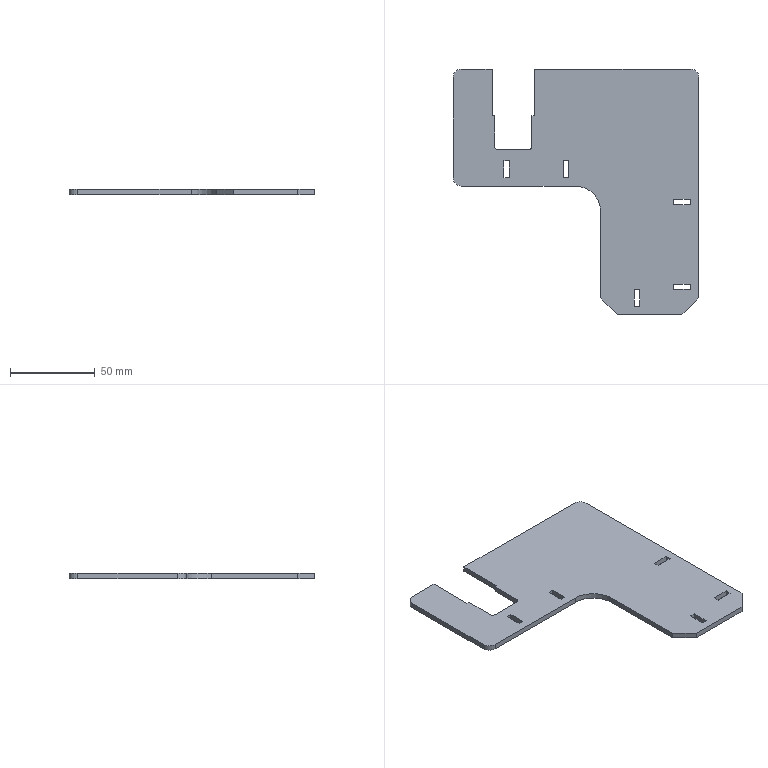Part | SolidWorks | features FlatPattern 1, SMBaseFlange 1, SheetMetal 1 | 1 solid | 44 faces | box 145 x 145 x 3.2 mm | volume 41790 mm3 | plane 38 | cylinder 6 | commonest cylinder face diameters 10 x3 4 x2 30 x1
STEP:
#1=CARTESIAN_POINT('',(-266.995,-106.198,3.2));
#2=VERTEX_POINT('',#1);
#3=CARTESIAN_POINT('',(-266.995,-133.698,3.2));
#4=VERTEX_POINT('',#3);
#5=CARTESIAN_POINT('',(-266.995,-133.698,3.2));
#6=DIRECTION('',(0.,-1.,0.));
#7=VECTOR('',#6,1000.);
#8=LINE('',#5,#7);
#9=EDGE_CURVE('',#2,#4,#8,.T.);
#10=ORIENTED_EDGE('',*,*,#9,.T.);
#11=CARTESIAN_POINT('',(-268.495,-133.698,3.2));
#12=VERTEX_POINT('',#11);
#13=CARTESIAN_POINT('',(-268.495,-133.698,3.2));
#14=DIRECTION('',(-1.,0.,0.));
#15=VECTOR('',#14,1000.);
#16=LINE('',#13,#15);
#17=EDGE_CURVE('',#4,#12,#16,.T.);
#18=ORIENTED_EDGE('',*,*,#17,.T.);
#19=CARTESIAN_POINT('',(-268.495,-151.698,3.2));
#20=VERTEX_POINT('',#19);
#21=CARTESIAN_POINT('',(-268.495,-151.698,3.2));
#22=DIRECTION('',(0.,-1.,0.));
#23=VECTOR('',#22,1000.);
#24=LINE('',#21,#23);
#25=EDGE_CURVE('',#12,#20,#24,.T.);
#26=ORIENTED_EDGE('',*,*,#25,.T.);
#27=CARTESIAN_POINT('',(-270.495,-153.698,3.2));
#28=VERTEX_POINT('',#27);
#29=CARTESIAN_POINT('',(-270.495,-151.698,3.2));
#30=DIRECTION('',(0.,0.,-1.));
#31=DIRECTION('',(1.,0.,0.));
#32=AXIS2_PLACEMENT_3D('',#29,#30,#31);
#33=CIRCLE('',#32,2.);
#34=EDGE_CURVE('',#20,#28,#33,.T.);
#35=ORIENTED_EDGE('',*,*,#34,.T.);
#36=CARTESIAN_POINT('',(-288.495,-153.698,3.2));
#37=VERTEX_POINT('',#36);
#38=CARTESIAN_POINT('',(-288.495,-153.698,3.2));
#39=DIRECTION('',(-1.,0.,0.));
#40=VECTOR('',#39,1000.);
#41=LINE('',#38,#40);
#42=EDGE_CURVE('',#28,#37,#41,.T.);
#43=ORIENTED_EDGE('',*,*,#42,.T.);
#44=CARTESIAN_POINT('',(-290.495,-151.698,3.2));
#45=VERTEX_POINT('',#44);
#46=CARTESIAN_POINT('',(-288.495,-151.698,3.2));
#47=DIRECTION('',(0.,0.,-1.));
#48=DIRECTION('',(1.,0.,0.));
#49=AXIS2_PLACEMENT_3D('',#46,#47,#48);
#50=CIRCLE('',#49,2.);
#51=EDGE_CURVE('',#37,#45,#50,.T.);
#52=ORIENTED_EDGE('',*,*,#51,.T.);
#53=CARTESIAN_POINT('',(-290.495,-133.698,3.2));
#54=VERTEX_POINT('',#53);
#55=CARTESIAN_POINT('',(-290.495,-133.698,3.2));
#56=DIRECTION('',(0.,1.,0.));
#57=VECTOR('',#56,1000.);
#58=LINE('',#55,#57);
#59=EDGE_CURVE('',#45,#54,#58,.T.);
#60=ORIENTED_EDGE('',*,*,#59,.T.);
#61=CARTESIAN_POINT('',(-291.995,-133.698,3.2));
#62=VERTEX_POINT('',#61);
#63=CARTESIAN_POINT('',(-291.995,-133.698,3.2));
#64=DIRECTION('',(-1.,0.,0.));
#65=VECTOR('',#64,1000.);
#66=LINE('',#63,#65);
#67=EDGE_CURVE('',#54,#62,#66,.T.);
#68=ORIENTED_EDGE('',*,*,#67,.T.);
#69=CARTESIAN_POINT('',(-291.995,-106.198,3.2));
#70=VERTEX_POINT('',#69);
#71=CARTESIAN_POINT('',(-291.995,-133.698,3.2));
#72=DIRECTION('',(0.,1.,0.));
#73=VECTOR('',#72,1000.);
#74=LINE('',#71,#73);
#75=EDGE_CURVE('',#62,#70,#74,.T.);
#76=ORIENTED_EDGE('',*,*,#75,.T.);
#77=CARTESIAN_POINT('',(-309.995,-106.198,3.2));
#78=VERTEX_POINT('',#77);
#79=CARTESIAN_POINT('',(-309.995,-106.198,3.2));
#80=DIRECTION('',(-1.,0.,0.));
#81=VECTOR('',#80,1000.);
#82=LINE('',#79,#81);
#83=EDGE_CURVE('',#70,#78,#82,.T.);
#84=ORIENTED_EDGE('',*,*,#83,.T.);
#85=CARTESIAN_POINT('',(-314.995,-111.198,3.2));
#86=VERTEX_POINT('',#85);
#87=CARTESIAN_POINT('',(-309.995,-111.198,3.2));
#88=DIRECTION('',(0.,0.,1.));
#89=DIRECTION('',(-1.,0.,0.));
#90=AXIS2_PLACEMENT_3D('',#87,#88,#89);
#91=CIRCLE('',#90,5.);
#92=EDGE_CURVE('',#78,#86,#91,.T.);
#93=ORIENTED_EDGE('',*,*,#92,.T.);
#94=CARTESIAN_POINT('',(-314.995,-170.198,3.2));
#95=VERTEX_POINT('',#94);
#96=CARTESIAN_POINT('',(-314.995,-170.198,3.2));
#97=DIRECTION('',(0.,-1.,0.));
#98=VECTOR('',#97,1000.);
#99=LINE('',#96,#98);
#100=EDGE_CURVE('',#86,#95,#99,.T.);
#101=ORIENTED_EDGE('',*,*,#100,.T.);
#102=CARTESIAN_POINT('',(-309.995,-175.198,3.2));
#103=VERTEX_POINT('',#102);
#104=CARTESIAN_POINT('',(-309.995,-170.198,3.2));
#105=DIRECTION('',(0.,0.,1.));
#106=DIRECTION('',(-1.,0.,0.));
#107=AXIS2_PLACEMENT_3D('',#104,#105,#106);
#108=CIRCLE('',#107,5.);
#109=EDGE_CURVE('',#95,#103,#108,.T.);
#110=ORIENTED_EDGE('',*,*,#109,.T.);
#111=CARTESIAN_POINT('',(-242.995,-175.198,3.2));
#112=VERTEX_POINT('',#111);
#113=CARTESIAN_POINT('',(-242.995,-175.198,3.2));
#114=DIRECTION('',(1.,0.,0.));
#115=VECTOR('',#114,1000.);
#116=LINE('',#113,#115);
#117=EDGE_CURVE('',#103,#112,#116,.T.);
#118=ORIENTED_EDGE('',*,*,#117,.T.);
#119=CARTESIAN_POINT('',(-227.995,-190.198,3.2));
#120=VERTEX_POINT('',#119);
#121=CARTESIAN_POINT('',(-242.995,-190.198,3.2));
#122=DIRECTION('',(0.,0.,-1.));
#123=DIRECTION('',(-1.,0.,0.));
#124=AXIS2_PLACEMENT_3D('',#121,#122,#123);
#125=CIRCLE('',#124,15.);
#126=EDGE_CURVE('',#112,#120,#125,.T.);
#127=ORIENTED_EDGE('',*,*,#126,.T.);
#128=CARTESIAN_POINT('',(-227.995,-241.198,3.2));
#129=VERTEX_POINT('',#128);
#130=CARTESIAN_POINT('',(-227.995,-241.198,3.2));
#131=DIRECTION('',(0.,-1.,0.));
#132=VECTOR('',#131,1000.);
#133=LINE('',#130,#132);
#134=EDGE_CURVE('',#120,#129,#133,.T.);
#135=ORIENTED_EDGE('',*,*,#134,.T.);
#136=CARTESIAN_POINT('',(-217.995,-251.198,3.2));
#137=VERTEX_POINT('',#136);
#138=CARTESIAN_POINT('',(-217.995,-251.198,3.2));
#139=DIRECTION('',(0.7071,-0.7071,0.));
#140=VECTOR('',#139,1000.);
#141=LINE('',#138,#140);
#142=EDGE_CURVE('',#129,#137,#141,.T.);
#143=ORIENTED_EDGE('',*,*,#142,.T.);
#144=CARTESIAN_POINT('',(-179.995,-251.198,3.2));
#145=VERTEX_POINT('',#144);
#146=CARTESIAN_POINT('',(-179.995,-251.198,3.2));
#147=DIRECTION('',(1.,0.,0.));
#148=VECTOR('',#147,1000.);
#149=LINE('',#146,#148);
#150=EDGE_CURVE('',#137,#145,#149,.T.);
#151=ORIENTED_EDGE('',*,*,#150,.T.);
#152=CARTESIAN_POINT('',(-169.995,-241.198,3.2));
#153=VERTEX_POINT('',#152);
#154=CARTESIAN_POINT('',(-169.995,-241.198,3.2));
#155=DIRECTION('',(0.7071,0.7071,0.));
#156=VECTOR('',#155,1000.);
#157=LINE('',#154,#156);
#158=EDGE_CURVE('',#145,#153,#157,.T.);
#159=ORIENTED_EDGE('',*,*,#158,.T.);
#160=CARTESIAN_POINT('',(-169.995,-111.198,3.2));
#161=VERTEX_POINT('',#160);
#162=CARTESIAN_POINT('',(-169.995,-241.198,3.2));
#163=DIRECTION('',(0.,1.,0.));
#164=VECTOR('',#163,1000.);
#165=LINE('',#162,#164);
#166=EDGE_CURVE('',#153,#161,#165,.T.);
#167=ORIENTED_EDGE('',*,*,#166,.T.);
#168=CARTESIAN_POINT('',(-174.995,-106.198,3.2));
#169=VERTEX_POINT('',#168);
#170=CARTESIAN_POINT('',(-174.995,-111.198,3.2));
#171=DIRECTION('',(0.,0.,1.));
#172=DIRECTION('',(1.,0.,0.));
#173=AXIS2_PLACEMENT_3D('',#170,#171,#172);
#174=CIRCLE('',#173,5.);
#175=EDGE_CURVE('',#161,#169,#174,.T.);
#176=ORIENTED_EDGE('',*,*,#175,.T.);
#177=CARTESIAN_POINT('',(-174.995,-106.198,3.2));
#178=DIRECTION('',(-1.,0.,0.));
#179=VECTOR('',#178,1000.);
#180=LINE('',#177,#179);
#181=EDGE_CURVE('',#169,#2,#180,.T.);
#182=ORIENTED_EDGE('',*,*,#181,.T.);
#183=EDGE_LOOP('',(#10,#18,#26,#35,#43,#52,#60,#68,#76,#84,#93,#101,#110,#118,#127,#135,#143,#151,#159,#167,#176,#182));
#184=FACE_OUTER_BOUND('',#183,.T.);
#185=CARTESIAN_POINT('',(-184.995,-236.198,3.2));
#186=VERTEX_POINT('',#185);
#187=CARTESIAN_POINT('',(-174.995,-236.198,3.2));
#188=VERTEX_POINT('',#187);
#189=CARTESIAN_POINT('',(-184.995,-236.198,3.2));
#190=DIRECTION('',(1.,0.,0.));
#191=VECTOR('',#190,1000.);
#192=LINE('',#189,#191);
#193=EDGE_CURVE('',#186,#188,#192,.T.);
#194=ORIENTED_EDGE('',*,*,#193,.F.);
#195=CARTESIAN_POINT('',(-184.995,-232.998,3.2));
#196=VERTEX_POINT('',#195);
#197=CARTESIAN_POINT('',(-184.995,-236.198,3.2));
#198=DIRECTION('',(0.,-1.,0.));
#199=VECTOR('',#198,1000.);
#200=LINE('',#197,#199);
#201=EDGE_CURVE('',#196,#186,#200,.T.);
#202=ORIENTED_EDGE('',*,*,#201,.F.);
#203=CARTESIAN_POINT('',(-174.995,-232.998,3.2));
#204=VERTEX_POINT('',#203);
#205=CARTESIAN_POINT('',(-184.995,-232.998,3.2));
#206=DIRECTION('',(-1.,0.,0.));
#207=VECTOR('',#206,1000.);
#208=LINE('',#205,#207);
#209=EDGE_CURVE('',#204,#196,#208,.T.);
#210=ORIENTED_EDGE('',*,*,#209,.F.);
#211=CARTESIAN_POINT('',(-174.995,-236.198,3.2));
#212=DIRECTION('',(0.,1.,0.));
#213=VECTOR('',#212,1000.);
#214=LINE('',#211,#213);
#215=EDGE_CURVE('',#188,#204,#214,.T.);
#216=ORIENTED_EDGE('',*,*,#215,.F.);
#217=EDGE_LOOP('',(#194,#202,#210,#216));
#218=FACE_BOUND('',#217,.T.);
#219=CARTESIAN_POINT('',(-174.995,-182.998,3.2));
#220=VERTEX_POINT('',#219);
#221=CARTESIAN_POINT('',(-184.995,-182.998,3.2));
#222=VERTEX_POINT('',#221);
#223=CARTESIAN_POINT('',(-174.995,-182.998,3.2));
#224=DIRECTION('',(-1.,0.,0.));
#225=VECTOR('',#224,1000.);
#226=LINE('',#223,#225);
#227=EDGE_CURVE('',#220,#222,#226,.T.);
#228=ORIENTED_EDGE('',*,*,#227,.F.);
#229=CARTESIAN_POINT('',(-174.995,-186.198,3.2));
#230=VERTEX_POINT('',#229);
#231=CARTESIAN_POINT('',(-174.995,-186.198,3.2));
#232=DIRECTION('',(0.,1.,0.));
#233=VECTOR('',#232,1000.);
#234=LINE('',#231,#233);
#235=EDGE_CURVE('',#230,#220,#234,.T.);
#236=ORIENTED_EDGE('',*,*,#235,.F.);
#237=CARTESIAN_POINT('',(-184.995,-186.198,3.2));
#238=VERTEX_POINT('',#237);
#239=CARTESIAN_POINT('',(-174.995,-186.198,3.2));
#240=DIRECTION('',(1.,0.,0.));
#241=VECTOR('',#240,1000.);
#242=LINE('',#239,#241);
#243=EDGE_CURVE('',#238,#230,#242,.T.);
#244=ORIENTED_EDGE('',*,*,#243,.F.);
#245=CARTESIAN_POINT('',(-184.995,-186.198,3.2));
#246=DIRECTION('',(0.,-1.,0.));
#247=VECTOR('',#246,1000.);
#248=LINE('',#245,#247);
#249=EDGE_CURVE('',#222,#238,#248,.T.);
#250=ORIENTED_EDGE('',*,*,#249,.F.);
#251=EDGE_LOOP('',(#228,#236,#244,#250));
#252=FACE_BOUND('',#251,.T.);
#253=CARTESIAN_POINT('',(-207.995,-246.198,3.2));
#254=VERTEX_POINT('',#253);
#255=CARTESIAN_POINT('',(-204.795,-246.198,3.2));
#256=VERTEX_POINT('',#255);
#257=CARTESIAN_POINT('',(-207.995,-246.198,3.2));
#258=DIRECTION('',(1.,0.,0.));
#259=VECTOR('',#258,1000.);
#260=LINE('',#257,#259);
#261=EDGE_CURVE('',#254,#256,#260,.T.);
#262=ORIENTED_EDGE('',*,*,#261,.F.);
#263=CARTESIAN_POINT('',(-207.995,-236.198,3.2));
#264=VERTEX_POINT('',#263);
#265=CARTESIAN_POINT('',(-207.995,-246.198,3.2));
#266=DIRECTION('',(0.,-1.,0.));
#267=VECTOR('',#266,1000.);
#268=LINE('',#265,#267);
#269=EDGE_CURVE('',#264,#254,#268,.T.);
#270=ORIENTED_EDGE('',*,*,#269,.F.);
#271=CARTESIAN_POINT('',(-204.795,-236.198,3.2));
#272=VERTEX_POINT('',#271);
#273=CARTESIAN_POINT('',(-207.995,-236.198,3.2));
#274=DIRECTION('',(-1.,0.,0.));
#275=VECTOR('',#274,1000.);
#276=LINE('',#273,#275);
#277=EDGE_CURVE('',#272,#264,#276,.T.);
#278=ORIENTED_EDGE('',*,*,#277,.F.);
#279=CARTESIAN_POINT('',(-204.795,-246.198,3.2));
#280=DIRECTION('',(0.,1.,0.));
#281=VECTOR('',#280,1000.);
#282=LINE('',#279,#281);
#283=EDGE_CURVE('',#256,#272,#282,.T.);
#284=ORIENTED_EDGE('',*,*,#283,.F.);
#285=EDGE_LOOP('',(#262,#270,#278,#284));
#286=FACE_BOUND('',#285,.T.);
#287=CARTESIAN_POINT('',(-249.995,-170.198,3.2));
#288=VERTEX_POINT('',#287);
#289=CARTESIAN_POINT('',(-246.795,-170.198,3.2));
#290=VERTEX_POINT('',#289);
#291=CARTESIAN_POINT('',(-249.995,-170.198,3.2));
#292=DIRECTION('',(1.,0.,0.));
#293=VECTOR('',#292,1000.);
#294=LINE('',#291,#293);
#295=EDGE_CURVE('',#288,#290,#294,.T.);
#296=ORIENTED_EDGE('',*,*,#295,.F.);
#297=CARTESIAN_POINT('',(-249.995,-160.198,3.2));
#298=VERTEX_POINT('',#297);
#299=CARTESIAN_POINT('',(-249.995,-160.198,3.2));
#300=DIRECTION('',(0.,-1.,0.));
#301=VECTOR('',#300,1000.);
#302=LINE('',#299,#301);
#303=EDGE_CURVE('',#298,#288,#302,.T.);
#304=ORIENTED_EDGE('',*,*,#303,.F.);
#305=CARTESIAN_POINT('',(-246.795,-160.198,3.2));
#306=VERTEX_POINT('',#305);
#307=CARTESIAN_POINT('',(-249.995,-160.198,3.2));
#308=DIRECTION('',(-1.,0.,0.));
#309=VECTOR('',#308,1000.);
#310=LINE('',#307,#309);
#311=EDGE_CURVE('',#306,#298,#310,.T.);
#312=ORIENTED_EDGE('',*,*,#311,.F.);
#313=CARTESIAN_POINT('',(-246.795,-160.198,3.2));
#314=DIRECTION('',(0.,1.,0.));
#315=VECTOR('',#314,1000.);
#316=LINE('',#313,#315);
#317=EDGE_CURVE('',#290,#306,#316,.T.);
#318=ORIENTED_EDGE('',*,*,#317,.F.);
#319=EDGE_LOOP('',(#296,#304,#312,#318));
#320=FACE_BOUND('',#319,.T.);
#321=CARTESIAN_POINT('',(-281.795,-160.198,3.2));
#322=VERTEX_POINT('',#321);
#323=CARTESIAN_POINT('',(-284.995,-160.198,3.2));
#324=VERTEX_POINT('',#323);
#325=CARTESIAN_POINT('',(-281.795,-160.198,3.2));
#326=DIRECTION('',(-1.,0.,0.));
#327=VECTOR('',#326,1000.);
#328=LINE('',#325,#327);
#329=EDGE_CURVE('',#322,#324,#328,.T.);
#330=ORIENTED_EDGE('',*,*,#329,.F.);
#331=CARTESIAN_POINT('',(-281.795,-170.198,3.2));
#332=VERTEX_POINT('',#331);
#333=CARTESIAN_POINT('',(-281.795,-170.198,3.2));
#334=DIRECTION('',(0.,1.,0.));
#335=VECTOR('',#334,1000.);
#336=LINE('',#333,#335);
#337=EDGE_CURVE('',#332,#322,#336,.T.);
#338=ORIENTED_EDGE('',*,*,#337,.F.);
#339=CARTESIAN_POINT('',(-284.995,-170.198,3.2));
#340=VERTEX_POINT('',#339);
#341=CARTESIAN_POINT('',(-281.795,-170.198,3.2));
#342=DIRECTION('',(1.,0.,0.));
#343=VECTOR('',#342,1000.);
#344=LINE('',#341,#343);
#345=EDGE_CURVE('',#340,#332,#344,.T.);
#346=ORIENTED_EDGE('',*,*,#345,.F.);
#347=CARTESIAN_POINT('',(-284.995,-170.198,3.2));
#348=DIRECTION('',(0.,-1.,0.));
#349=VECTOR('',#348,1000.);
#350=LINE('',#347,#349);
#351=EDGE_CURVE('',#324,#340,#350,.T.);
#352=ORIENTED_EDGE('',*,*,#351,.F.);
#353=EDGE_LOOP('',(#330,#338,#346,#352));
#354=FACE_BOUND('',#353,.T.);
#355=CARTESIAN_POINT('',(-174.995,-111.198,3.2));
#356=DIRECTION('',(0.,0.,1.));
#357=DIRECTION('',(1.,0.,0.));
#358=AXIS2_PLACEMENT_3D('',#355,#356,#357);
#359=PLANE('',#358);
#360=ADVANCED_FACE('',(#184,#218,#252,#286,#320,#354),#359,.T.);
#361=CARTESIAN_POINT('',(-249.995,-160.198,0.));
#362=VERTEX_POINT('',#361);
#363=CARTESIAN_POINT('',(-249.995,-170.198,0.));
#364=VERTEX_POINT('',#363);
#365=CARTESIAN_POINT('',(-249.995,-160.198,0.));
#366=DIRECTION('',(0.,-1.,0.));
#367=VECTOR('',#366,1000.);
#368=LINE('',#365,#367);
#369=EDGE_CURVE('',#362,#364,#368,.T.);
#370=ORIENTED_EDGE('',*,*,#369,.T.);
#371=CARTESIAN_POINT('',(-246.795,-170.198,0.));
#372=VERTEX_POINT('',#371);
#373=CARTESIAN_POINT('',(-249.995,-170.198,0.));
#374=DIRECTION('',(1.,0.,0.));
#375=VECTOR('',#374,1000.);
#376=LINE('',#373,#375);
#377=EDGE_CURVE('',#364,#372,#376,.T.);
#378=ORIENTED_EDGE('',*,*,#377,.T.);
#379=CARTESIAN_POINT('',(-246.795,-160.198,0.));
#380=VERTEX_POINT('',#379);
#381=CARTESIAN_POINT('',(-246.795,-160.198,0.));
#382=DIRECTION('',(0.,1.,0.));
#383=VECTOR('',#382,1000.);
#384=LINE('',#381,#383);
#385=EDGE_CURVE('',#372,#380,#384,.T.);
#386=ORIENTED_EDGE('',*,*,#385,.T.);
#387=CARTESIAN_POINT('',(-249.995,-160.198,0.));
#388=DIRECTION('',(-1.,0.,0.));
#389=VECTOR('',#388,1000.);
#390=LINE('',#387,#389);
#391=EDGE_CURVE('',#380,#362,#390,.T.);
#392=ORIENTED_EDGE('',*,*,#391,.T.);
#393=EDGE_LOOP('',(#370,#378,#386,#392));
#394=FACE_BOUND('',#393,.T.);
#395=CARTESIAN_POINT('',(-174.995,-186.198,0.));
#396=VERTEX_POINT('',#395);
#397=CARTESIAN_POINT('',(-174.995,-182.998,0.));
#398=VERTEX_POINT('',#397);
#399=CARTESIAN_POINT('',(-174.995,-186.198,0.));
#400=DIRECTION('',(0.,1.,0.));
#401=VECTOR('',#400,1000.);
#402=LINE('',#399,#401);
#403=EDGE_CURVE('',#396,#398,#402,.T.);
#404=ORIENTED_EDGE('',*,*,#403,.T.);
#405=CARTESIAN_POINT('',(-184.995,-182.998,0.));
#406=VERTEX_POINT('',#405);
#407=CARTESIAN_POINT('',(-174.995,-182.998,0.));
#408=DIRECTION('',(-1.,0.,0.));
#409=VECTOR('',#408,1000.);
#410=LINE('',#407,#409);
#411=EDGE_CURVE('',#398,#406,#410,.T.);
#412=ORIENTED_EDGE('',*,*,#411,.T.);
#413=CARTESIAN_POINT('',(-184.995,-186.198,0.));
#414=VERTEX_POINT('',#413);
#415=CARTESIAN_POINT('',(-184.995,-186.198,0.));
#416=DIRECTION('',(0.,-1.,0.));
#417=VECTOR('',#416,1000.);
#418=LINE('',#415,#417);
#419=EDGE_CURVE('',#406,#414,#418,.T.);
#420=ORIENTED_EDGE('',*,*,#419,.T.);
#421=CARTESIAN_POINT('',(-174.995,-186.198,0.));
#422=DIRECTION('',(1.,0.,0.));
#423=VECTOR('',#422,1000.);
#424=LINE('',#421,#423);
#425=EDGE_CURVE('',#414,#396,#424,.T.);
#426=ORIENTED_EDGE('',*,*,#425,.T.);
#427=EDGE_LOOP('',(#404,#412,#420,#426));
#428=FACE_BOUND('',#427,.T.);
#429=CARTESIAN_POINT('',(-266.995,-106.198,0.));
#430=VERTEX_POINT('',#429);
#431=CARTESIAN_POINT('',(-266.995,-133.698,0.));
#432=VERTEX_POINT('',#431);
#433=CARTESIAN_POINT('',(-266.995,-133.698,0.));
#434=DIRECTION('',(0.,-1.,0.));
#435=VECTOR('',#434,1000.);
#436=LINE('',#433,#435);
#437=EDGE_CURVE('',#430,#432,#436,.T.);
#438=ORIENTED_EDGE('',*,*,#437,.F.);
#439=CARTESIAN_POINT('',(-174.995,-106.198,0.));
#440=VERTEX_POINT('',#439);
#441=CARTESIAN_POINT('',(-174.995,-106.198,0.));
#442=DIRECTION('',(-1.,0.,0.));
#443=VECTOR('',#442,1000.);
#444=LINE('',#441,#443);
#445=EDGE_CURVE('',#440,#430,#444,.T.);
#446=ORIENTED_EDGE('',*,*,#445,.F.);
#447=CARTESIAN_POINT('',(-169.995,-111.198,0.));
#448=VERTEX_POINT('',#447);
#449=CARTESIAN_POINT('',(-174.995,-111.198,0.));
#450=DIRECTION('',(0.,0.,1.));
#451=DIRECTION('',(1.,0.,0.));
#452=AXIS2_PLACEMENT_3D('',#449,#450,#451);
#453=CIRCLE('',#452,5.);
#454=EDGE_CURVE('',#448,#440,#453,.T.);
#455=ORIENTED_EDGE('',*,*,#454,.F.);
#456=CARTESIAN_POINT('',(-169.995,-241.198,0.));
#457=VERTEX_POINT('',#456);
#458=CARTESIAN_POINT('',(-169.995,-241.198,0.));
#459=DIRECTION('',(0.,1.,0.));
#460=VECTOR('',#459,1000.);
#461=LINE('',#458,#460);
#462=EDGE_CURVE('',#457,#448,#461,.T.);
#463=ORIENTED_EDGE('',*,*,#462,.F.);
#464=CARTESIAN_POINT('',(-179.995,-251.198,0.));
#465=VERTEX_POINT('',#464);
#466=CARTESIAN_POINT('',(-169.995,-241.198,0.));
#467=DIRECTION('',(0.7071,0.7071,0.));
#468=VECTOR('',#467,1000.);
#469=LINE('',#466,#468);
#470=EDGE_CURVE('',#465,#457,#469,.T.);
#471=ORIENTED_EDGE('',*,*,#470,.F.);
#472=CARTESIAN_POINT('',(-217.995,-251.198,0.));
#473=VERTEX_POINT('',#472);
#474=CARTESIAN_POINT('',(-179.995,-251.198,0.));
#475=DIRECTION('',(1.,0.,0.));
#476=VECTOR('',#475,1000.);
#477=LINE('',#474,#476);
#478=EDGE_CURVE('',#473,#465,#477,.T.);
#479=ORIENTED_EDGE('',*,*,#478,.F.);
#480=CARTESIAN_POINT('',(-227.995,-241.198,0.));
#481=VERTEX_POINT('',#480);
#482=CARTESIAN_POINT('',(-217.995,-251.198,0.));
#483=DIRECTION('',(0.7071,-0.7071,0.));
#484=VECTOR('',#483,1000.);
#485=LINE('',#482,#484);
#486=EDGE_CURVE('',#481,#473,#485,.T.);
#487=ORIENTED_EDGE('',*,*,#486,.F.);
#488=CARTESIAN_POINT('',(-227.995,-190.198,0.));
#489=VERTEX_POINT('',#488);
#490=CARTESIAN_POINT('',(-227.995,-241.198,0.));
#491=DIRECTION('',(0.,-1.,0.));
#492=VECTOR('',#491,1000.);
#493=LINE('',#490,#492);
#494=EDGE_CURVE('',#489,#481,#493,.T.);
#495=ORIENTED_EDGE('',*,*,#494,.F.);
#496=CARTESIAN_POINT('',(-242.995,-175.198,0.));
#497=VERTEX_POINT('',#496);
#498=CARTESIAN_POINT('',(-242.995,-190.198,0.));
#499=DIRECTION('',(0.,0.,-1.));
#500=DIRECTION('',(-1.,0.,0.));
#501=AXIS2_PLACEMENT_3D('',#498,#499,#500);
#502=CIRCLE('',#501,15.);
#503=EDGE_CURVE('',#497,#489,#502,.T.);
#504=ORIENTED_EDGE('',*,*,#503,.F.);
#505=CARTESIAN_POINT('',(-309.995,-175.198,0.));
#506=VERTEX_POINT('',#505);
#507=CARTESIAN_POINT('',(-242.995,-175.198,0.));
#508=DIRECTION('',(1.,0.,0.));
#509=VECTOR('',#508,1000.);
#510=LINE('',#507,#509);
#511=EDGE_CURVE('',#506,#497,#510,.T.);
#512=ORIENTED_EDGE('',*,*,#511,.F.);
#513=CARTESIAN_POINT('',(-314.995,-170.198,0.));
#514=VERTEX_POINT('',#513);
#515=CARTESIAN_POINT('',(-309.995,-170.198,0.));
#516=DIRECTION('',(0.,0.,1.));
#517=DIRECTION('',(-1.,0.,0.));
#518=AXIS2_PLACEMENT_3D('',#515,#516,#517);
#519=CIRCLE('',#518,5.);
#520=EDGE_CURVE('',#514,#506,#519,.T.);
#521=ORIENTED_EDGE('',*,*,#520,.F.);
#522=CARTESIAN_POINT('',(-314.995,-111.198,0.));
#523=VERTEX_POINT('',#522);
#524=CARTESIAN_POINT('',(-314.995,-170.198,0.));
#525=DIRECTION('',(0.,-1.,0.));
#526=VECTOR('',#525,1000.);
#527=LINE('',#524,#526);
#528=EDGE_CURVE('',#523,#514,#527,.T.);
#529=ORIENTED_EDGE('',*,*,#528,.F.);
#530=CARTESIAN_POINT('',(-309.995,-106.198,0.));
#531=VERTEX_POINT('',#530);
#532=CARTESIAN_POINT('',(-309.995,-111.198,0.));
#533=DIRECTION('',(0.,0.,1.));
#534=DIRECTION('',(-1.,0.,0.));
#535=AXIS2_PLACEMENT_3D('',#532,#533,#534);
#536=CIRCLE('',#535,5.);
#537=EDGE_CURVE('',#531,#523,#536,.T.);
#538=ORIENTED_EDGE('',*,*,#537,.F.);
#539=CARTESIAN_POINT('',(-291.995,-106.198,0.));
#540=VERTEX_POINT('',#539);
#541=CARTESIAN_POINT('',(-309.995,-106.198,0.));
#542=DIRECTION('',(-1.,0.,0.));
#543=VECTOR('',#542,1000.);
#544=LINE('',#541,#543);
#545=EDGE_CURVE('',#540,#531,#544,.T.);
#546=ORIENTED_EDGE('',*,*,#545,.F.);
#547=CARTESIAN_POINT('',(-291.995,-133.698,0.));
#548=VERTEX_POINT('',#547);
#549=CARTESIAN_POINT('',(-291.995,-133.698,0.));
#550=DIRECTION('',(0.,1.,0.));
#551=VECTOR('',#550,1000.);
#552=LINE('',#549,#551);
#553=EDGE_CURVE('',#548,#540,#552,.T.);
#554=ORIENTED_EDGE('',*,*,#553,.F.);
#555=CARTESIAN_POINT('',(-290.495,-133.698,0.));
#556=VERTEX_POINT('',#555);
#557=CARTESIAN_POINT('',(-291.995,-133.698,0.));
#558=DIRECTION('',(-1.,0.,0.));
#559=VECTOR('',#558,1000.);
#560=LINE('',#557,#559);
#561=EDGE_CURVE('',#556,#548,#560,.T.);
#562=ORIENTED_EDGE('',*,*,#561,.F.);
#563=CARTESIAN_POINT('',(-290.495,-151.698,0.));
#564=VERTEX_POINT('',#563);
#565=CARTESIAN_POINT('',(-290.495,-133.698,0.));
#566=DIRECTION('',(0.,1.,0.));
#567=VECTOR('',#566,1000.);
#568=LINE('',#565,#567);
#569=EDGE_CURVE('',#564,#556,#568,.T.);
#570=ORIENTED_EDGE('',*,*,#569,.F.);
#571=CARTESIAN_POINT('',(-288.495,-153.698,0.));
#572=VERTEX_POINT('',#571);
#573=CARTESIAN_POINT('',(-288.495,-151.698,0.));
#574=DIRECTION('',(0.,0.,-1.));
#575=DIRECTION('',(1.,0.,0.));
#576=AXIS2_PLACEMENT_3D('',#573,#574,#575);
#577=CIRCLE('',#576,2.);
#578=EDGE_CURVE('',#572,#564,#577,.T.);
#579=ORIENTED_EDGE('',*,*,#578,.F.);
#580=CARTESIAN_POINT('',(-270.495,-153.698,0.));
#581=VERTEX_POINT('',#580);
#582=CARTESIAN_POINT('',(-288.495,-153.698,0.));
#583=DIRECTION('',(-1.,0.,0.));
#584=VECTOR('',#583,1000.);
#585=LINE('',#582,#584);
#586=EDGE_CURVE('',#581,#572,#585,.T.);
#587=ORIENTED_EDGE('',*,*,#586,.F.);
#588=CARTESIAN_POINT('',(-268.495,-151.698,0.));
#589=VERTEX_POINT('',#588);
#590=CARTESIAN_POINT('',(-270.495,-151.698,0.));
#591=DIRECTION('',(0.,0.,-1.));
#592=DIRECTION('',(1.,0.,0.));
#593=AXIS2_PLACEMENT_3D('',#590,#591,#592);
#594=CIRCLE('',#593,2.);
#595=EDGE_CURVE('',#589,#581,#594,.T.);
#596=ORIENTED_EDGE('',*,*,#595,.F.);
#597=CARTESIAN_POINT('',(-268.495,-133.698,0.));
#598=VERTEX_POINT('',#597);
#599=CARTESIAN_POINT('',(-268.495,-151.698,0.));
#600=DIRECTION('',(0.,-1.,0.));
#601=VECTOR('',#600,1000.);
#602=LINE('',#599,#601);
#603=EDGE_CURVE('',#598,#589,#602,.T.);
#604=ORIENTED_EDGE('',*,*,#603,.F.);
#605=CARTESIAN_POINT('',(-268.495,-133.698,0.));
#606=DIRECTION('',(-1.,0.,0.));
#607=VECTOR('',#606,1000.);
#608=LINE('',#605,#607);
#609=EDGE_CURVE('',#432,#598,#608,.T.);
#610=ORIENTED_EDGE('',*,*,#609,.F.);
#611=EDGE_LOOP('',(#438,#446,#455,#463,#471,#479,#487,#495,#504,#512,#521,#529,#538,#546,#554,#562,#570,#579,#587,#596,#604,#610));
#612=FACE_OUTER_BOUND('',#611,.T.);
#613=CARTESIAN_POINT('',(-184.995,-232.998,0.));
#614=VERTEX_POINT('',#613);
#615=CARTESIAN_POINT('',(-184.995,-236.198,0.));
#616=VERTEX_POINT('',#615);
#617=CARTESIAN_POINT('',(-184.995,-236.198,0.));
#618=DIRECTION('',(0.,-1.,0.));
#619=VECTOR('',#618,1000.);
#620=LINE('',#617,#619);
#621=EDGE_CURVE('',#614,#616,#620,.T.);
#622=ORIENTED_EDGE('',*,*,#621,.T.);
#623=CARTESIAN_POINT('',(-174.995,-236.198,0.));
#624=VERTEX_POINT('',#623);
#625=CARTESIAN_POINT('',(-184.995,-236.198,0.));
#626=DIRECTION('',(1.,0.,0.));
#627=VECTOR('',#626,1000.);
#628=LINE('',#625,#627);
#629=EDGE_CURVE('',#616,#624,#628,.T.);
#630=ORIENTED_EDGE('',*,*,#629,.T.);
#631=CARTESIAN_POINT('',(-174.995,-232.998,0.));
#632=VERTEX_POINT('',#631);
#633=CARTESIAN_POINT('',(-174.995,-236.198,0.));
#634=DIRECTION('',(0.,1.,0.));
#635=VECTOR('',#634,1000.);
#636=LINE('',#633,#635);
#637=EDGE_CURVE('',#624,#632,#636,.T.);
#638=ORIENTED_EDGE('',*,*,#637,.T.);
#639=CARTESIAN_POINT('',(-184.995,-232.998,0.));
#640=DIRECTION('',(-1.,0.,0.));
#641=VECTOR('',#640,1000.);
#642=LINE('',#639,#641);
#643=EDGE_CURVE('',#632,#614,#642,.T.);
#644=ORIENTED_EDGE('',*,*,#643,.T.);
#645=EDGE_LOOP('',(#622,#630,#638,#644));
#646=FACE_BOUND('',#645,.T.);
#647=CARTESIAN_POINT('',(-207.995,-236.198,0.));
#648=VERTEX_POINT('',#647);
#649=CARTESIAN_POINT('',(-207.995,-246.198,0.));
#650=VERTEX_POINT('',#649);
#651=CARTESIAN_POINT('',(-207.995,-246.198,0.));
#652=DIRECTION('',(0.,-1.,0.));
#653=VECTOR('',#652,1000.);
#654=LINE('',#651,#653);
#655=EDGE_CURVE('',#648,#650,#654,.T.);
#656=ORIENTED_EDGE('',*,*,#655,.T.);
#657=CARTESIAN_POINT('',(-204.795,-246.198,0.));
#658=VERTEX_POINT('',#657);
#659=CARTESIAN_POINT('',(-207.995,-246.198,0.));
#660=DIRECTION('',(1.,0.,0.));
#661=VECTOR('',#660,1000.);
#662=LINE('',#659,#661);
#663=EDGE_CURVE('',#650,#658,#662,.T.);
#664=ORIENTED_EDGE('',*,*,#663,.T.);
#665=CARTESIAN_POINT('',(-204.795,-236.198,0.));
#666=VERTEX_POINT('',#665);
#667=CARTESIAN_POINT('',(-204.795,-246.198,0.));
#668=DIRECTION('',(0.,1.,0.));
#669=VECTOR('',#668,1000.);
#670=LINE('',#667,#669);
#671=EDGE_CURVE('',#658,#666,#670,.T.);
#672=ORIENTED_EDGE('',*,*,#671,.T.);
#673=CARTESIAN_POINT('',(-207.995,-236.198,0.));
#674=DIRECTION('',(-1.,0.,0.));
#675=VECTOR('',#674,1000.);
#676=LINE('',#673,#675);
#677=EDGE_CURVE('',#666,#648,#676,.T.);
#678=ORIENTED_EDGE('',*,*,#677,.T.);
#679=EDGE_LOOP('',(#656,#664,#672,#678));
#680=FACE_BOUND('',#679,.T.);
#681=CARTESIAN_POINT('',(-281.795,-170.198,0.));
#682=VERTEX_POINT('',#681);
#683=CARTESIAN_POINT('',(-281.795,-160.198,0.));
#684=VERTEX_POINT('',#683);
#685=CARTESIAN_POINT('',(-281.795,-170.198,0.));
#686=DIRECTION('',(0.,1.,0.));
#687=VECTOR('',#686,1000.);
#688=LINE('',#685,#687);
#689=EDGE_CURVE('',#682,#684,#688,.T.);
#690=ORIENTED_EDGE('',*,*,#689,.T.);
#691=CARTESIAN_POINT('',(-284.995,-160.198,0.));
#692=VERTEX_POINT('',#691);
#693=CARTESIAN_POINT('',(-281.795,-160.198,0.));
#694=DIRECTION('',(-1.,0.,0.));
#695=VECTOR('',#694,1000.);
#696=LINE('',#693,#695);
#697=EDGE_CURVE('',#684,#692,#696,.T.);
#698=ORIENTED_EDGE('',*,*,#697,.T.);
#699=CARTESIAN_POINT('',(-284.995,-170.198,0.));
#700=VERTEX_POINT('',#699);
#701=CARTESIAN_POINT('',(-284.995,-170.198,0.));
#702=DIRECTION('',(0.,-1.,0.));
#703=VECTOR('',#702,1000.);
#704=LINE('',#701,#703);
#705=EDGE_CURVE('',#692,#700,#704,.T.);
#706=ORIENTED_EDGE('',*,*,#705,.T.);
#707=CARTESIAN_POINT('',(-281.795,-170.198,0.));
#708=DIRECTION('',(1.,0.,0.));
#709=VECTOR('',#708,1000.);
#710=LINE('',#707,#709);
#711=EDGE_CURVE('',#700,#682,#710,.T.);
#712=ORIENTED_EDGE('',*,*,#711,.T.);
#713=EDGE_LOOP('',(#690,#698,#706,#712));
#714=FACE_BOUND('',#713,.T.);
#715=CARTESIAN_POINT('',(-174.995,-111.198,0.));
#716=DIRECTION('',(0.,0.,1.));
#717=DIRECTION('',(1.,0.,0.));
#718=AXIS2_PLACEMENT_3D('',#715,#716,#717);
#719=PLANE('',#718);
#720=ADVANCED_FACE('',(#394,#428,#612,#646,#680,#714),#719,.F.);
#721=ORIENTED_EDGE('',*,*,#437,.T.);
#722=CARTESIAN_POINT('',(-266.995,-133.698,3.2));
#723=DIRECTION('',(0.,0.,-1.));
#724=VECTOR('',#723,1000.);
#725=LINE('',#722,#724);
#726=EDGE_CURVE('',#4,#432,#725,.T.);
#727=ORIENTED_EDGE('',*,*,#726,.F.);
#728=ORIENTED_EDGE('',*,*,#9,.F.);
#729=CARTESIAN_POINT('',(-266.995,-106.198,3.2));
#730=DIRECTION('',(0.,0.,-1.));
#731=VECTOR('',#730,1000.);
#732=LINE('',#729,#731);
#733=EDGE_CURVE('',#2,#430,#732,.T.);
#734=ORIENTED_EDGE('',*,*,#733,.T.);
#735=EDGE_LOOP('',(#721,#727,#728,#734));
#736=FACE_OUTER_BOUND('',#735,.T.);
#737=CARTESIAN_POINT('',(-266.995,-133.698,3.2));
#738=DIRECTION('',(1.,0.,0.));
#739=DIRECTION('',(0.,0.,-1.));
#740=AXIS2_PLACEMENT_3D('',#737,#738,#739);
#741=PLANE('',#740);
#742=ADVANCED_FACE('',(#736),#741,.F.);
#743=ORIENTED_EDGE('',*,*,#609,.T.);
#744=CARTESIAN_POINT('',(-268.495,-133.698,3.2));
#745=DIRECTION('',(0.,0.,-1.));
#746=VECTOR('',#745,1000.);
#747=LINE('',#744,#746);
#748=EDGE_CURVE('',#12,#598,#747,.T.);
#749=ORIENTED_EDGE('',*,*,#748,.F.);
#750=ORIENTED_EDGE('',*,*,#17,.F.);
#751=ORIENTED_EDGE('',*,*,#726,.T.);
#752=EDGE_LOOP('',(#743,#749,#750,#751));
#753=FACE_OUTER_BOUND('',#752,.T.);
#754=CARTESIAN_POINT('',(-268.495,-133.698,3.2));
#755=DIRECTION('',(0.,-1.,0.));
#756=DIRECTION('',(1.,0.,0.));
#757=AXIS2_PLACEMENT_3D('',#754,#755,#756);
#758=PLANE('',#757);
#759=ADVANCED_FACE('',(#753),#758,.F.);
#760=ORIENTED_EDGE('',*,*,#603,.T.);
#761=CARTESIAN_POINT('',(-268.495,-151.698,3.2));
#762=DIRECTION('',(0.,0.,-1.));
#763=VECTOR('',#762,1000.);
#764=LINE('',#761,#763);
#765=EDGE_CURVE('',#20,#589,#764,.T.);
#766=ORIENTED_EDGE('',*,*,#765,.F.);
#767=ORIENTED_EDGE('',*,*,#25,.F.);
#768=ORIENTED_EDGE('',*,*,#748,.T.);
#769=EDGE_LOOP('',(#760,#766,#767,#768));
#770=FACE_OUTER_BOUND('',#769,.T.);
#771=CARTESIAN_POINT('',(-268.495,-151.698,3.2));
#772=DIRECTION('',(1.,0.,0.));
#773=DIRECTION('',(0.,0.,-1.));
#774=AXIS2_PLACEMENT_3D('',#771,#772,#773);
#775=PLANE('',#774);
#776=ADVANCED_FACE('',(#770),#775,.F.);
#777=ORIENTED_EDGE('',*,*,#595,.T.);
#778=CARTESIAN_POINT('',(-270.495,-153.698,3.2));
#779=DIRECTION('',(0.,0.,-1.));
#780=VECTOR('',#779,1000.);
#781=LINE('',#778,#780);
#782=EDGE_CURVE('',#28,#581,#781,.T.);
#783=ORIENTED_EDGE('',*,*,#782,.F.);
#784=ORIENTED_EDGE('',*,*,#34,.F.);
#785=ORIENTED_EDGE('',*,*,#765,.T.);
#786=EDGE_LOOP('',(#777,#783,#784,#785));
#787=FACE_OUTER_BOUND('',#786,.T.);
#788=CARTESIAN_POINT('',(-270.495,-151.698,3.2));
#789=DIRECTION('',(0.,0.,-1.));
#790=DIRECTION('',(-1.,0.,0.));
#791=AXIS2_PLACEMENT_3D('',#788,#789,#790);
#792=CYLINDRICAL_SURFACE('',#791,2.);
#793=ADVANCED_FACE('',(#787),#792,.F.);
#794=ORIENTED_EDGE('',*,*,#586,.T.);
#795=CARTESIAN_POINT('',(-288.495,-153.698,3.2));
#796=DIRECTION('',(0.,0.,-1.));
#797=VECTOR('',#796,1000.);
#798=LINE('',#795,#797);
#799=EDGE_CURVE('',#37,#572,#798,.T.);
#800=ORIENTED_EDGE('',*,*,#799,.F.);
#801=ORIENTED_EDGE('',*,*,#42,.F.);
#802=ORIENTED_EDGE('',*,*,#782,.T.);
#803=EDGE_LOOP('',(#794,#800,#801,#802));
#804=FACE_OUTER_BOUND('',#803,.T.);
#805=CARTESIAN_POINT('',(-288.495,-153.698,3.2));
#806=DIRECTION('',(0.,-1.,0.));
#807=DIRECTION('',(0.,0.,-1.));
#808=AXIS2_PLACEMENT_3D('',#805,#806,#807);
#809=PLANE('',#808);
#810=ADVANCED_FACE('',(#804),#809,.F.);
#811=ORIENTED_EDGE('',*,*,#578,.T.);
#812=CARTESIAN_POINT('',(-290.495,-151.698,3.2));
#813=DIRECTION('',(0.,0.,-1.));
#814=VECTOR('',#813,1000.);
#815=LINE('',#812,#814);
#816=EDGE_CURVE('',#45,#564,#815,.T.);
#817=ORIENTED_EDGE('',*,*,#816,.F.);
#818=ORIENTED_EDGE('',*,*,#51,.F.);
#819=ORIENTED_EDGE('',*,*,#799,.T.);
#820=EDGE_LOOP('',(#811,#817,#818,#819));
#821=FACE_OUTER_BOUND('',#820,.T.);
#822=CARTESIAN_POINT('',(-288.495,-151.698,3.2));
#823=DIRECTION('',(0.,0.,-1.));
#824=DIRECTION('',(-1.,0.,0.));
#825=AXIS2_PLACEMENT_3D('',#822,#823,#824);
#826=CYLINDRICAL_SURFACE('',#825,2.);
#827=ADVANCED_FACE('',(#821),#826,.F.);
#828=ORIENTED_EDGE('',*,*,#569,.T.);
#829=CARTESIAN_POINT('',(-290.495,-133.698,3.2));
#830=DIRECTION('',(0.,0.,-1.));
#831=VECTOR('',#830,1000.);
#832=LINE('',#829,#831);
#833=EDGE_CURVE('',#54,#556,#832,.T.);
#834=ORIENTED_EDGE('',*,*,#833,.F.);
#835=ORIENTED_EDGE('',*,*,#59,.F.);
#836=ORIENTED_EDGE('',*,*,#816,.T.);
#837=EDGE_LOOP('',(#828,#834,#835,#836));
#838=FACE_OUTER_BOUND('',#837,.T.);
#839=CARTESIAN_POINT('',(-290.495,-133.698,3.2));
#840=DIRECTION('',(-1.,0.,0.));
#841=DIRECTION('',(0.,0.,1.));
#842=AXIS2_PLACEMENT_3D('',#839,#840,#841);
#843=PLANE('',#842);
#844=ADVANCED_FACE('',(#838),#843,.F.);
#845=ORIENTED_EDGE('',*,*,#561,.T.);
#846=CARTESIAN_POINT('',(-291.995,-133.698,3.2));
#847=DIRECTION('',(0.,0.,-1.));
#848=VECTOR('',#847,1000.);
#849=LINE('',#846,#848);
#850=EDGE_CURVE('',#62,#548,#849,.T.);
#851=ORIENTED_EDGE('',*,*,#850,.F.);
#852=ORIENTED_EDGE('',*,*,#67,.F.);
#853=ORIENTED_EDGE('',*,*,#833,.T.);
#854=EDGE_LOOP('',(#845,#851,#852,#853));
#855=FACE_OUTER_BOUND('',#854,.T.);
#856=CARTESIAN_POINT('',(-291.995,-133.698,3.2));
#857=DIRECTION('',(0.,-1.,0.));
#858=DIRECTION('',(0.,0.,-1.));
#859=AXIS2_PLACEMENT_3D('',#856,#857,#858);
#860=PLANE('',#859);
#861=ADVANCED_FACE('',(#855),#860,.F.);
#862=ORIENTED_EDGE('',*,*,#553,.T.);
#863=CARTESIAN_POINT('',(-291.995,-106.198,3.2));
#864=DIRECTION('',(0.,0.,-1.));
#865=VECTOR('',#864,1000.);
#866=LINE('',#863,#865);
#867=EDGE_CURVE('',#70,#540,#866,.T.);
#868=ORIENTED_EDGE('',*,*,#867,.F.);
#869=ORIENTED_EDGE('',*,*,#75,.F.);
#870=ORIENTED_EDGE('',*,*,#850,.T.);
#871=EDGE_LOOP('',(#862,#868,#869,#870));
#872=FACE_OUTER_BOUND('',#871,.T.);
#873=CARTESIAN_POINT('',(-291.995,-133.698,3.2));
#874=DIRECTION('',(-1.,0.,0.));
#875=DIRECTION('',(0.,0.,1.));
#876=AXIS2_PLACEMENT_3D('',#873,#874,#875);
#877=PLANE('',#876);
#878=ADVANCED_FACE('',(#872),#877,.F.);
#879=ORIENTED_EDGE('',*,*,#545,.T.);
#880=CARTESIAN_POINT('',(-309.995,-106.198,3.2));
#881=DIRECTION('',(0.,0.,-1.));
#882=VECTOR('',#881,1000.);
#883=LINE('',#880,#882);
#884=EDGE_CURVE('',#78,#531,#883,.T.);
#885=ORIENTED_EDGE('',*,*,#884,.F.);
#886=ORIENTED_EDGE('',*,*,#83,.F.);
#887=ORIENTED_EDGE('',*,*,#867,.T.);
#888=EDGE_LOOP('',(#879,#885,#886,#887));
#889=FACE_OUTER_BOUND('',#888,.T.);
#890=CARTESIAN_POINT('',(-309.995,-106.198,3.2));
#891=DIRECTION('',(0.,-1.,0.));
#892=DIRECTION('',(0.,0.,-1.));
#893=AXIS2_PLACEMENT_3D('',#890,#891,#892);
#894=PLANE('',#893);
#895=ADVANCED_FACE('',(#889),#894,.F.);
#896=ORIENTED_EDGE('',*,*,#537,.T.);
#897=CARTESIAN_POINT('',(-314.995,-111.198,3.2));
#898=DIRECTION('',(0.,0.,-1.));
#899=VECTOR('',#898,1000.);
#900=LINE('',#897,#899);
#901=EDGE_CURVE('',#86,#523,#900,.T.);
#902=ORIENTED_EDGE('',*,*,#901,.F.);
#903=ORIENTED_EDGE('',*,*,#92,.F.);
#904=ORIENTED_EDGE('',*,*,#884,.T.);
#905=EDGE_LOOP('',(#896,#902,#903,#904));
#906=FACE_OUTER_BOUND('',#905,.T.);
#907=CARTESIAN_POINT('',(-309.995,-111.198,3.2));
#908=DIRECTION('',(0.,0.,-1.));
#909=DIRECTION('',(-1.,0.,0.));
#910=AXIS2_PLACEMENT_3D('',#907,#908,#909);
#911=CYLINDRICAL_SURFACE('',#910,5.);
#912=ADVANCED_FACE('',(#906),#911,.T.);
#913=ORIENTED_EDGE('',*,*,#528,.T.);
#914=CARTESIAN_POINT('',(-314.995,-170.198,3.2));
#915=DIRECTION('',(0.,0.,-1.));
#916=VECTOR('',#915,1000.);
#917=LINE('',#914,#916);
#918=EDGE_CURVE('',#95,#514,#917,.T.);
#919=ORIENTED_EDGE('',*,*,#918,.F.);
#920=ORIENTED_EDGE('',*,*,#100,.F.);
#921=ORIENTED_EDGE('',*,*,#901,.T.);
#922=EDGE_LOOP('',(#913,#919,#920,#921));
#923=FACE_OUTER_BOUND('',#922,.T.);
#924=CARTESIAN_POINT('',(-314.995,-170.198,3.2));
#925=DIRECTION('',(1.,0.,0.));
#926=DIRECTION('',(0.,0.,-1.));
#927=AXIS2_PLACEMENT_3D('',#924,#925,#926);
#928=PLANE('',#927);
#929=ADVANCED_FACE('',(#923),#928,.F.);
#930=ORIENTED_EDGE('',*,*,#520,.T.);
#931=CARTESIAN_POINT('',(-309.995,-175.198,3.2));
#932=DIRECTION('',(0.,0.,-1.));
#933=VECTOR('',#932,1000.);
#934=LINE('',#931,#933);
#935=EDGE_CURVE('',#103,#506,#934,.T.);
#936=ORIENTED_EDGE('',*,*,#935,.F.);
#937=ORIENTED_EDGE('',*,*,#109,.F.);
#938=ORIENTED_EDGE('',*,*,#918,.T.);
#939=EDGE_LOOP('',(#930,#936,#937,#938));
#940=FACE_OUTER_BOUND('',#939,.T.);
#941=CARTESIAN_POINT('',(-309.995,-170.198,3.2));
#942=DIRECTION('',(0.,0.,-1.));
#943=DIRECTION('',(-1.,0.,0.));
#944=AXIS2_PLACEMENT_3D('',#941,#942,#943);
#945=CYLINDRICAL_SURFACE('',#944,5.);
#946=ADVANCED_FACE('',(#940),#945,.T.);
#947=ORIENTED_EDGE('',*,*,#511,.T.);
#948=CARTESIAN_POINT('',(-242.995,-175.198,3.2));
#949=DIRECTION('',(0.,0.,-1.));
#950=VECTOR('',#949,1000.);
#951=LINE('',#948,#950);
#952=EDGE_CURVE('',#112,#497,#951,.T.);
#953=ORIENTED_EDGE('',*,*,#952,.F.);
#954=ORIENTED_EDGE('',*,*,#117,.F.);
#955=ORIENTED_EDGE('',*,*,#935,.T.);
#956=EDGE_LOOP('',(#947,#953,#954,#955));
#957=FACE_OUTER_BOUND('',#956,.T.);
#958=CARTESIAN_POINT('',(-242.995,-175.198,3.2));
#959=DIRECTION('',(0.,1.,0.));
#960=DIRECTION('',(0.,0.,1.));
#961=AXIS2_PLACEMENT_3D('',#958,#959,#960);
#962=PLANE('',#961);
#963=ADVANCED_FACE('',(#957),#962,.F.);
#964=ORIENTED_EDGE('',*,*,#503,.T.);
#965=CARTESIAN_POINT('',(-227.995,-190.198,3.2));
#966=DIRECTION('',(0.,0.,-1.));
#967=VECTOR('',#966,1000.);
#968=LINE('',#965,#967);
#969=EDGE_CURVE('',#120,#489,#968,.T.);
#970=ORIENTED_EDGE('',*,*,#969,.F.);
#971=ORIENTED_EDGE('',*,*,#126,.F.);
#972=ORIENTED_EDGE('',*,*,#952,.T.);
#973=EDGE_LOOP('',(#964,#970,#971,#972));
#974=FACE_OUTER_BOUND('',#973,.T.);
#975=CARTESIAN_POINT('',(-242.995,-190.198,3.2));
#976=DIRECTION('',(0.,0.,-1.));
#977=DIRECTION('',(-1.,0.,0.));
#978=AXIS2_PLACEMENT_3D('',#975,#976,#977);
#979=CYLINDRICAL_SURFACE('',#978,15.);
#980=ADVANCED_FACE('',(#974),#979,.F.);
#981=ORIENTED_EDGE('',*,*,#494,.T.);
#982=CARTESIAN_POINT('',(-227.995,-241.198,3.2));
#983=DIRECTION('',(0.,0.,-1.));
#984=VECTOR('',#983,1000.);
#985=LINE('',#982,#984);
#986=EDGE_CURVE('',#129,#481,#985,.T.);
#987=ORIENTED_EDGE('',*,*,#986,.F.);
#988=ORIENTED_EDGE('',*,*,#134,.F.);
#989=ORIENTED_EDGE('',*,*,#969,.T.);
#990=EDGE_LOOP('',(#981,#987,#988,#989));
#991=FACE_OUTER_BOUND('',#990,.T.);
#992=CARTESIAN_POINT('',(-227.995,-241.198,3.2));
#993=DIRECTION('',(1.,0.,0.));
#994=DIRECTION('',(0.,1.,0.));
#995=AXIS2_PLACEMENT_3D('',#992,#993,#994);
#996=PLANE('',#995);
#997=ADVANCED_FACE('',(#991),#996,.F.);
#998=ORIENTED_EDGE('',*,*,#486,.T.);
#999=CARTESIAN_POINT('',(-217.995,-251.198,3.2));
#1000=DIRECTION('',(0.,0.,-1.));
#1001=VECTOR('',#1000,1000.);
#1002=LINE('',#999,#1001);
#1003=EDGE_CURVE('',#137,#473,#1002,.T.);
#1004=ORIENTED_EDGE('',*,*,#1003,.F.);
#1005=ORIENTED_EDGE('',*,*,#142,.F.);
#1006=ORIENTED_EDGE('',*,*,#986,.T.);
#1007=EDGE_LOOP('',(#998,#1004,#1005,#1006));
#1008=FACE_OUTER_BOUND('',#1007,.T.);
#1009=CARTESIAN_POINT('',(-217.995,-251.198,3.2));
#1010=DIRECTION('',(0.7071,0.7071,0.));
#1011=DIRECTION('',(-0.7071,0.7071,0.));
#1012=AXIS2_PLACEMENT_3D('',#1009,#1010,#1011);
#1013=PLANE('',#1012);
#1014=ADVANCED_FACE('',(#1008),#1013,.F.);
#1015=ORIENTED_EDGE('',*,*,#478,.T.);
#1016=CARTESIAN_POINT('',(-179.995,-251.198,3.2));
#1017=DIRECTION('',(0.,0.,-1.));
#1018=VECTOR('',#1017,1000.);
#1019=LINE('',#1016,#1018);
#1020=EDGE_CURVE('',#145,#465,#1019,.T.);
#1021=ORIENTED_EDGE('',*,*,#1020,.F.);
#1022=ORIENTED_EDGE('',*,*,#150,.F.);
#1023=ORIENTED_EDGE('',*,*,#1003,.T.);
#1024=EDGE_LOOP('',(#1015,#1021,#1022,#1023));
#1025=FACE_OUTER_BOUND('',#1024,.T.);
#1026=CARTESIAN_POINT('',(-179.995,-251.198,3.2));
#1027=DIRECTION('',(0.,1.,0.));
#1028=DIRECTION('',(0.,0.,1.));
#1029=AXIS2_PLACEMENT_3D('',#1026,#1027,#1028);
#1030=PLANE('',#1029);
#1031=ADVANCED_FACE('',(#1025),#1030,.F.);
#1032=ORIENTED_EDGE('',*,*,#470,.T.);
#1033=CARTESIAN_POINT('',(-169.995,-241.198,3.2));
#1034=DIRECTION('',(0.,0.,-1.));
#1035=VECTOR('',#1034,1000.);
#1036=LINE('',#1033,#1035);
#1037=EDGE_CURVE('',#153,#457,#1036,.T.);
#1038=ORIENTED_EDGE('',*,*,#1037,.F.);
#1039=ORIENTED_EDGE('',*,*,#158,.F.);
#1040=ORIENTED_EDGE('',*,*,#1020,.T.);
#1041=EDGE_LOOP('',(#1032,#1038,#1039,#1040));
#1042=FACE_OUTER_BOUND('',#1041,.T.);
#1043=CARTESIAN_POINT('',(-169.995,-241.198,3.2));
#1044=DIRECTION('',(-0.7071,0.7071,0.));
#1045=DIRECTION('',(-0.7071,-0.7071,0.));
#1046=AXIS2_PLACEMENT_3D('',#1043,#1044,#1045);
#1047=PLANE('',#1046);
#1048=ADVANCED_FACE('',(#1042),#1047,.F.);
#1049=ORIENTED_EDGE('',*,*,#462,.T.);
#1050=CARTESIAN_POINT('',(-169.995,-111.198,3.2));
#1051=DIRECTION('',(0.,0.,-1.));
#1052=VECTOR('',#1051,1000.);
#1053=LINE('',#1050,#1052);
#1054=EDGE_CURVE('',#161,#448,#1053,.T.);
#1055=ORIENTED_EDGE('',*,*,#1054,.F.);
#1056=ORIENTED_EDGE('',*,*,#166,.F.);
#1057=ORIENTED_EDGE('',*,*,#1037,.T.);
#1058=EDGE_LOOP('',(#1049,#1055,#1056,#1057));
#1059=FACE_OUTER_BOUND('',#1058,.T.);
#1060=CARTESIAN_POINT('',(-169.995,-241.198,3.2));
#1061=DIRECTION('',(-1.,0.,0.));
#1062=DIRECTION('',(0.,0.,1.));
#1063=AXIS2_PLACEMENT_3D('',#1060,#1061,#1062);
#1064=PLANE('',#1063);
#1065=ADVANCED_FACE('',(#1059),#1064,.F.);
#1066=ORIENTED_EDGE('',*,*,#454,.T.);
#1067=CARTESIAN_POINT('',(-174.995,-106.198,3.2));
#1068=DIRECTION('',(0.,0.,-1.));
#1069=VECTOR('',#1068,1000.);
#1070=LINE('',#1067,#1069);
#1071=EDGE_CURVE('',#169,#440,#1070,.T.);
#1072=ORIENTED_EDGE('',*,*,#1071,.F.);
#1073=ORIENTED_EDGE('',*,*,#175,.F.);
#1074=ORIENTED_EDGE('',*,*,#1054,.T.);
#1075=EDGE_LOOP('',(#1066,#1072,#1073,#1074));
#1076=FACE_OUTER_BOUND('',#1075,.T.);
#1077=CARTESIAN_POINT('',(-174.995,-111.198,3.2));
#1078=DIRECTION('',(0.,0.,-1.));
#1079=DIRECTION('',(-1.,0.,0.));
#1080=AXIS2_PLACEMENT_3D('',#1077,#1078,#1079);
#1081=CYLINDRICAL_SURFACE('',#1080,5.);
#1082=ADVANCED_FACE('',(#1076),#1081,.T.);
#1083=ORIENTED_EDGE('',*,*,#445,.T.);
#1084=ORIENTED_EDGE('',*,*,#733,.F.);
#1085=ORIENTED_EDGE('',*,*,#181,.F.);
#1086=ORIENTED_EDGE('',*,*,#1071,.T.);
#1087=EDGE_LOOP('',(#1083,#1084,#1085,#1086));
#1088=FACE_OUTER_BOUND('',#1087,.T.);
#1089=CARTESIAN_POINT('',(-174.995,-106.198,3.2));
#1090=DIRECTION('',(0.,-1.,0.));
#1091=DIRECTION('',(1.,0.,0.));
#1092=AXIS2_PLACEMENT_3D('',#1089,#1090,#1091);
#1093=PLANE('',#1092);
#1094=ADVANCED_FACE('',(#1088),#1093,.F.);
#1095=ORIENTED_EDGE('',*,*,#621,.F.);
#1096=CARTESIAN_POINT('',(-184.995,-232.998,3.2));
#1097=DIRECTION('',(0.,0.,-1.));
#1098=VECTOR('',#1097,1000.);
#1099=LINE('',#1096,#1098);
#1100=EDGE_CURVE('',#196,#614,#1099,.T.);
#1101=ORIENTED_EDGE('',*,*,#1100,.F.);
#1102=ORIENTED_EDGE('',*,*,#201,.T.);
#1103=CARTESIAN_POINT('',(-184.995,-236.198,3.2));
#1104=DIRECTION('',(0.,0.,-1.));
#1105=VECTOR('',#1104,1000.);
#1106=LINE('',#1103,#1105);
#1107=EDGE_CURVE('',#186,#616,#1106,.T.);
#1108=ORIENTED_EDGE('',*,*,#1107,.T.);
#1109=EDGE_LOOP('',(#1095,#1101,#1102,#1108));
#1110=FACE_OUTER_BOUND('',#1109,.T.);
#1111=CARTESIAN_POINT('',(-184.995,-236.198,3.2));
#1112=DIRECTION('',(1.,0.,0.));
#1113=DIRECTION('',(0.,0.,-1.));
#1114=AXIS2_PLACEMENT_3D('',#1111,#1112,#1113);
#1115=PLANE('',#1114);
#1116=ADVANCED_FACE('',(#1110),#1115,.T.);
#1117=ORIENTED_EDGE('',*,*,#629,.F.);
#1118=ORIENTED_EDGE('',*,*,#1107,.F.);
#1119=ORIENTED_EDGE('',*,*,#193,.T.);
#1120=CARTESIAN_POINT('',(-174.995,-236.198,3.2));
#1121=DIRECTION('',(0.,0.,-1.));
#1122=VECTOR('',#1121,1000.);
#1123=LINE('',#1120,#1122);
#1124=EDGE_CURVE('',#188,#624,#1123,.T.);
#1125=ORIENTED_EDGE('',*,*,#1124,.T.);
#1126=EDGE_LOOP('',(#1117,#1118,#1119,#1125));
#1127=FACE_OUTER_BOUND('',#1126,.T.);
#1128=CARTESIAN_POINT('',(-184.995,-236.198,3.2));
#1129=DIRECTION('',(0.,1.,0.));
#1130=DIRECTION('',(0.,0.,1.));
#1131=AXIS2_PLACEMENT_3D('',#1128,#1129,#1130);
#1132=PLANE('',#1131);
#1133=ADVANCED_FACE('',(#1127),#1132,.T.);
#1134=ORIENTED_EDGE('',*,*,#637,.F.);
#1135=ORIENTED_EDGE('',*,*,#1124,.F.);
#1136=ORIENTED_EDGE('',*,*,#215,.T.);
#1137=CARTESIAN_POINT('',(-174.995,-232.998,3.2));
#1138=DIRECTION('',(0.,0.,-1.));
#1139=VECTOR('',#1138,1000.);
#1140=LINE('',#1137,#1139);
#1141=EDGE_CURVE('',#204,#632,#1140,.T.);
#1142=ORIENTED_EDGE('',*,*,#1141,.T.);
#1143=EDGE_LOOP('',(#1134,#1135,#1136,#1142));
#1144=FACE_OUTER_BOUND('',#1143,.T.);
#1145=CARTESIAN_POINT('',(-174.995,-236.198,3.2));
#1146=DIRECTION('',(-1.,0.,0.));
#1147=DIRECTION('',(0.,0.,1.));
#1148=AXIS2_PLACEMENT_3D('',#1145,#1146,#1147);
#1149=PLANE('',#1148);
#1150=ADVANCED_FACE('',(#1144),#1149,.T.);
#1151=ORIENTED_EDGE('',*,*,#643,.F.);
#1152=ORIENTED_EDGE('',*,*,#1141,.F.);
#1153=ORIENTED_EDGE('',*,*,#209,.T.);
#1154=ORIENTED_EDGE('',*,*,#1100,.T.);
#1155=EDGE_LOOP('',(#1151,#1152,#1153,#1154));
#1156=FACE_OUTER_BOUND('',#1155,.T.);
#1157=CARTESIAN_POINT('',(-184.995,-232.998,3.2));
#1158=DIRECTION('',(0.,-1.,0.));
#1159=DIRECTION('',(0.,0.,-1.));
#1160=AXIS2_PLACEMENT_3D('',#1157,#1158,#1159);
#1161=PLANE('',#1160);
#1162=ADVANCED_FACE('',(#1156),#1161,.T.);
#1163=ORIENTED_EDGE('',*,*,#403,.F.);
#1164=CARTESIAN_POINT('',(-174.995,-186.198,3.2));
#1165=DIRECTION('',(0.,0.,-1.));
#1166=VECTOR('',#1165,1000.);
#1167=LINE('',#1164,#1166);
#1168=EDGE_CURVE('',#230,#396,#1167,.T.);
#1169=ORIENTED_EDGE('',*,*,#1168,.F.);
#1170=ORIENTED_EDGE('',*,*,#235,.T.);
#1171=CARTESIAN_POINT('',(-174.995,-182.998,3.2));
#1172=DIRECTION('',(0.,0.,-1.));
#1173=VECTOR('',#1172,1000.);
#1174=LINE('',#1171,#1173);
#1175=EDGE_CURVE('',#220,#398,#1174,.T.);
#1176=ORIENTED_EDGE('',*,*,#1175,.T.);
#1177=EDGE_LOOP('',(#1163,#1169,#1170,#1176));
#1178=FACE_OUTER_BOUND('',#1177,.T.);
#1179=CARTESIAN_POINT('',(-174.995,-186.198,3.2));
#1180=DIRECTION('',(-1.,0.,0.));
#1181=DIRECTION('',(0.,0.,1.));
#1182=AXIS2_PLACEMENT_3D('',#1179,#1180,#1181);
#1183=PLANE('',#1182);
#1184=ADVANCED_FACE('',(#1178),#1183,.T.);
#1185=ORIENTED_EDGE('',*,*,#411,.F.);
#1186=ORIENTED_EDGE('',*,*,#1175,.F.);
#1187=ORIENTED_EDGE('',*,*,#227,.T.);
#1188=CARTESIAN_POINT('',(-184.995,-182.998,3.2));
#1189=DIRECTION('',(0.,0.,-1.));
#1190=VECTOR('',#1189,1000.);
#1191=LINE('',#1188,#1190);
#1192=EDGE_CURVE('',#222,#406,#1191,.T.);
#1193=ORIENTED_EDGE('',*,*,#1192,.T.);
#1194=EDGE_LOOP('',(#1185,#1186,#1187,#1193));
#1195=FACE_OUTER_BOUND('',#1194,.T.);
#1196=CARTESIAN_POINT('',(-174.995,-182.998,3.2));
#1197=DIRECTION('',(0.,-1.,0.));
#1198=DIRECTION('',(0.,0.,-1.));
#1199=AXIS2_PLACEMENT_3D('',#1196,#1197,#1198);
#1200=PLANE('',#1199);
#1201=ADVANCED_FACE('',(#1195),#1200,.T.);
#1202=ORIENTED_EDGE('',*,*,#419,.F.);
#1203=ORIENTED_EDGE('',*,*,#1192,.F.);
#1204=ORIENTED_EDGE('',*,*,#249,.T.);
#1205=CARTESIAN_POINT('',(-184.995,-186.198,3.2));
#1206=DIRECTION('',(0.,0.,-1.));
#1207=VECTOR('',#1206,1000.);
#1208=LINE('',#1205,#1207);
#1209=EDGE_CURVE('',#238,#414,#1208,.T.);
#1210=ORIENTED_EDGE('',*,*,#1209,.T.);
#1211=EDGE_LOOP('',(#1202,#1203,#1204,#1210));
#1212=FACE_OUTER_BOUND('',#1211,.T.);
#1213=CARTESIAN_POINT('',(-184.995,-186.198,3.2));
#1214=DIRECTION('',(1.,0.,0.));
#1215=DIRECTION('',(0.,0.,-1.));
#1216=AXIS2_PLACEMENT_3D('',#1213,#1214,#1215);
#1217=PLANE('',#1216);
#1218=ADVANCED_FACE('',(#1212),#1217,.T.);
#1219=ORIENTED_EDGE('',*,*,#425,.F.);
#1220=ORIENTED_EDGE('',*,*,#1209,.F.);
#1221=ORIENTED_EDGE('',*,*,#243,.T.);
#1222=ORIENTED_EDGE('',*,*,#1168,.T.);
#1223=EDGE_LOOP('',(#1219,#1220,#1221,#1222));
#1224=FACE_OUTER_BOUND('',#1223,.T.);
#1225=CARTESIAN_POINT('',(-174.995,-186.198,3.2));
#1226=DIRECTION('',(0.,1.,0.));
#1227=DIRECTION('',(0.,0.,1.));
#1228=AXIS2_PLACEMENT_3D('',#1225,#1226,#1227);
#1229=PLANE('',#1228);
#1230=ADVANCED_FACE('',(#1224),#1229,.T.);
#1231=ORIENTED_EDGE('',*,*,#655,.F.);
#1232=CARTESIAN_POINT('',(-207.995,-236.198,3.2));
#1233=DIRECTION('',(0.,0.,-1.));
#1234=VECTOR('',#1233,1000.);
#1235=LINE('',#1232,#1234);
#1236=EDGE_CURVE('',#264,#648,#1235,.T.);
#1237=ORIENTED_EDGE('',*,*,#1236,.F.);
#1238=ORIENTED_EDGE('',*,*,#269,.T.);
#1239=CARTESIAN_POINT('',(-207.995,-246.198,3.2));
#1240=DIRECTION('',(0.,0.,-1.));
#1241=VECTOR('',#1240,1000.);
#1242=LINE('',#1239,#1241);
#1243=EDGE_CURVE('',#254,#650,#1242,.T.);
#1244=ORIENTED_EDGE('',*,*,#1243,.T.);
#1245=EDGE_LOOP('',(#1231,#1237,#1238,#1244));
#1246=FACE_OUTER_BOUND('',#1245,.T.);
#1247=CARTESIAN_POINT('',(-207.995,-246.198,3.2));
#1248=DIRECTION('',(1.,0.,0.));
#1249=DIRECTION('',(0.,0.,-1.));
#1250=AXIS2_PLACEMENT_3D('',#1247,#1248,#1249);
#1251=PLANE('',#1250);
#1252=ADVANCED_FACE('',(#1246),#1251,.T.);
#1253=ORIENTED_EDGE('',*,*,#663,.F.);
#1254=ORIENTED_EDGE('',*,*,#1243,.F.);
#1255=ORIENTED_EDGE('',*,*,#261,.T.);
#1256=CARTESIAN_POINT('',(-204.795,-246.198,3.2));
#1257=DIRECTION('',(0.,0.,-1.));
#1258=VECTOR('',#1257,1000.);
#1259=LINE('',#1256,#1258);
#1260=EDGE_CURVE('',#256,#658,#1259,.T.);
#1261=ORIENTED_EDGE('',*,*,#1260,.T.);
#1262=EDGE_LOOP('',(#1253,#1254,#1255,#1261));
#1263=FACE_OUTER_BOUND('',#1262,.T.);
#1264=CARTESIAN_POINT('',(-207.995,-246.198,3.2));
#1265=DIRECTION('',(0.,1.,0.));
#1266=DIRECTION('',(0.,0.,1.));
#1267=AXIS2_PLACEMENT_3D('',#1264,#1265,#1266);
#1268=PLANE('',#1267);
#1269=ADVANCED_FACE('',(#1263),#1268,.T.);
#1270=ORIENTED_EDGE('',*,*,#671,.F.);
#1271=ORIENTED_EDGE('',*,*,#1260,.F.);
#1272=ORIENTED_EDGE('',*,*,#283,.T.);
#1273=CARTESIAN_POINT('',(-204.795,-236.198,3.2));
#1274=DIRECTION('',(0.,0.,-1.));
#1275=VECTOR('',#1274,1000.);
#1276=LINE('',#1273,#1275);
#1277=EDGE_CURVE('',#272,#666,#1276,.T.);
#1278=ORIENTED_EDGE('',*,*,#1277,.T.);
#1279=EDGE_LOOP('',(#1270,#1271,#1272,#1278));
#1280=FACE_OUTER_BOUND('',#1279,.T.);
#1281=CARTESIAN_POINT('',(-204.795,-246.198,3.2));
#1282=DIRECTION('',(-1.,0.,0.));
#1283=DIRECTION('',(0.,0.,1.));
#1284=AXIS2_PLACEMENT_3D('',#1281,#1282,#1283);
#1285=PLANE('',#1284);
#1286=ADVANCED_FACE('',(#1280),#1285,.T.);
#1287=ORIENTED_EDGE('',*,*,#677,.F.);
#1288=ORIENTED_EDGE('',*,*,#1277,.F.);
#1289=ORIENTED_EDGE('',*,*,#277,.T.);
#1290=ORIENTED_EDGE('',*,*,#1236,.T.);
#1291=EDGE_LOOP('',(#1287,#1288,#1289,#1290));
#1292=FACE_OUTER_BOUND('',#1291,.T.);
#1293=CARTESIAN_POINT('',(-207.995,-236.198,3.2));
#1294=DIRECTION('',(0.,-1.,0.));
#1295=DIRECTION('',(0.,0.,-1.));
#1296=AXIS2_PLACEMENT_3D('',#1293,#1294,#1295);
#1297=PLANE('',#1296);
#1298=ADVANCED_FACE('',(#1292),#1297,.T.);
#1299=ORIENTED_EDGE('',*,*,#369,.F.);
#1300=CARTESIAN_POINT('',(-249.995,-160.198,3.2));
#1301=DIRECTION('',(0.,0.,-1.));
#1302=VECTOR('',#1301,1000.);
#1303=LINE('',#1300,#1302);
#1304=EDGE_CURVE('',#298,#362,#1303,.T.);
#1305=ORIENTED_EDGE('',*,*,#1304,.F.);
#1306=ORIENTED_EDGE('',*,*,#303,.T.);
#1307=CARTESIAN_POINT('',(-249.995,-170.198,3.2));
#1308=DIRECTION('',(0.,0.,-1.));
#1309=VECTOR('',#1308,1000.);
#1310=LINE('',#1307,#1309);
#1311=EDGE_CURVE('',#288,#364,#1310,.T.);
#1312=ORIENTED_EDGE('',*,*,#1311,.T.);
#1313=EDGE_LOOP('',(#1299,#1305,#1306,#1312));
#1314=FACE_OUTER_BOUND('',#1313,.T.);
#1315=CARTESIAN_POINT('',(-249.995,-160.198,3.2));
#1316=DIRECTION('',(1.,0.,0.));
#1317=DIRECTION('',(0.,0.,-1.));
#1318=AXIS2_PLACEMENT_3D('',#1315,#1316,#1317);
#1319=PLANE('',#1318);
#1320=ADVANCED_FACE('',(#1314),#1319,.T.);
#1321=ORIENTED_EDGE('',*,*,#377,.F.);
#1322=ORIENTED_EDGE('',*,*,#1311,.F.);
#1323=ORIENTED_EDGE('',*,*,#295,.T.);
#1324=CARTESIAN_POINT('',(-246.795,-170.198,3.2));
#1325=DIRECTION('',(0.,0.,-1.));
#1326=VECTOR('',#1325,1000.);
#1327=LINE('',#1324,#1326);
#1328=EDGE_CURVE('',#290,#372,#1327,.T.);
#1329=ORIENTED_EDGE('',*,*,#1328,.T.);
#1330=EDGE_LOOP('',(#1321,#1322,#1323,#1329));
#1331=FACE_OUTER_BOUND('',#1330,.T.);
#1332=CARTESIAN_POINT('',(-249.995,-170.198,3.2));
#1333=DIRECTION('',(0.,1.,0.));
#1334=DIRECTION('',(0.,0.,1.));
#1335=AXIS2_PLACEMENT_3D('',#1332,#1333,#1334);
#1336=PLANE('',#1335);
#1337=ADVANCED_FACE('',(#1331),#1336,.T.);
#1338=ORIENTED_EDGE('',*,*,#385,.F.);
#1339=ORIENTED_EDGE('',*,*,#1328,.F.);
#1340=ORIENTED_EDGE('',*,*,#317,.T.);
#1341=CARTESIAN_POINT('',(-246.795,-160.198,3.2));
#1342=DIRECTION('',(0.,0.,-1.));
#1343=VECTOR('',#1342,1000.);
#1344=LINE('',#1341,#1343);
#1345=EDGE_CURVE('',#306,#380,#1344,.T.);
#1346=ORIENTED_EDGE('',*,*,#1345,.T.);
#1347=EDGE_LOOP('',(#1338,#1339,#1340,#1346));
#1348=FACE_OUTER_BOUND('',#1347,.T.);
#1349=CARTESIAN_POINT('',(-246.795,-160.198,3.2));
#1350=DIRECTION('',(-1.,0.,0.));
#1351=DIRECTION('',(0.,0.,1.));
#1352=AXIS2_PLACEMENT_3D('',#1349,#1350,#1351);
#1353=PLANE('',#1352);
#1354=ADVANCED_FACE('',(#1348),#1353,.T.);
#1355=ORIENTED_EDGE('',*,*,#391,.F.);
#1356=ORIENTED_EDGE('',*,*,#1345,.F.);
#1357=ORIENTED_EDGE('',*,*,#311,.T.);
#1358=ORIENTED_EDGE('',*,*,#1304,.T.);
#1359=EDGE_LOOP('',(#1355,#1356,#1357,#1358));
#1360=FACE_OUTER_BOUND('',#1359,.T.);
#1361=CARTESIAN_POINT('',(-249.995,-160.198,3.2));
#1362=DIRECTION('',(0.,-1.,0.));
#1363=DIRECTION('',(0.,0.,-1.));
#1364=AXIS2_PLACEMENT_3D('',#1361,#1362,#1363);
#1365=PLANE('',#1364);
#1366=ADVANCED_FACE('',(#1360),#1365,.T.);
#1367=ORIENTED_EDGE('',*,*,#689,.F.);
#1368=CARTESIAN_POINT('',(-281.795,-170.198,3.2));
#1369=DIRECTION('',(0.,0.,-1.));
#1370=VECTOR('',#1369,1000.);
#1371=LINE('',#1368,#1370);
#1372=EDGE_CURVE('',#332,#682,#1371,.T.);
#1373=ORIENTED_EDGE('',*,*,#1372,.F.);
#1374=ORIENTED_EDGE('',*,*,#337,.T.);
#1375=CARTESIAN_POINT('',(-281.795,-160.198,3.2));
#1376=DIRECTION('',(0.,0.,-1.));
#1377=VECTOR('',#1376,1000.);
#1378=LINE('',#1375,#1377);
#1379=EDGE_CURVE('',#322,#684,#1378,.T.);
#1380=ORIENTED_EDGE('',*,*,#1379,.T.);
#1381=EDGE_LOOP('',(#1367,#1373,#1374,#1380));
#1382=FACE_OUTER_BOUND('',#1381,.T.);
#1383=CARTESIAN_POINT('',(-281.795,-170.198,3.2));
#1384=DIRECTION('',(-1.,0.,0.));
#1385=DIRECTION('',(0.,0.,1.));
#1386=AXIS2_PLACEMENT_3D('',#1383,#1384,#1385);
#1387=PLANE('',#1386);
#1388=ADVANCED_FACE('',(#1382),#1387,.T.);
#1389=ORIENTED_EDGE('',*,*,#697,.F.);
#1390=ORIENTED_EDGE('',*,*,#1379,.F.);
#1391=ORIENTED_EDGE('',*,*,#329,.T.);
#1392=CARTESIAN_POINT('',(-284.995,-160.198,3.2));
#1393=DIRECTION('',(0.,0.,-1.));
#1394=VECTOR('',#1393,1000.);
#1395=LINE('',#1392,#1394);
#1396=EDGE_CURVE('',#324,#692,#1395,.T.);
#1397=ORIENTED_EDGE('',*,*,#1396,.T.);
#1398=EDGE_LOOP('',(#1389,#1390,#1391,#1397));
#1399=FACE_OUTER_BOUND('',#1398,.T.);
#1400=CARTESIAN_POINT('',(-281.795,-160.198,3.2));
#1401=DIRECTION('',(0.,-1.,0.));
#1402=DIRECTION('',(0.,0.,-1.));
#1403=AXIS2_PLACEMENT_3D('',#1400,#1401,#1402);
#1404=PLANE('',#1403);
#1405=ADVANCED_FACE('',(#1399),#1404,.T.);
#1406=ORIENTED_EDGE('',*,*,#705,.F.);
#1407=ORIENTED_EDGE('',*,*,#1396,.F.);
#1408=ORIENTED_EDGE('',*,*,#351,.T.);
#1409=CARTESIAN_POINT('',(-284.995,-170.198,3.2));
#1410=DIRECTION('',(0.,0.,-1.));
#1411=VECTOR('',#1410,1000.);
#1412=LINE('',#1409,#1411);
#1413=EDGE_CURVE('',#340,#700,#1412,.T.);
#1414=ORIENTED_EDGE('',*,*,#1413,.T.);
#1415=EDGE_LOOP('',(#1406,#1407,#1408,#1414));
#1416=FACE_OUTER_BOUND('',#1415,.T.);
#1417=CARTESIAN_POINT('',(-284.995,-170.198,3.2));
#1418=DIRECTION('',(1.,0.,0.));
#1419=DIRECTION('',(0.,0.,-1.));
#1420=AXIS2_PLACEMENT_3D('',#1417,#1418,#1419);
#1421=PLANE('',#1420);
#1422=ADVANCED_FACE('',(#1416),#1421,.T.);
#1423=ORIENTED_EDGE('',*,*,#711,.F.);
#1424=ORIENTED_EDGE('',*,*,#1413,.F.);
#1425=ORIENTED_EDGE('',*,*,#345,.T.);
#1426=ORIENTED_EDGE('',*,*,#1372,.T.);
#1427=EDGE_LOOP('',(#1423,#1424,#1425,#1426));
#1428=FACE_OUTER_BOUND('',#1427,.T.);
#1429=CARTESIAN_POINT('',(-281.795,-170.198,3.2));
#1430=DIRECTION('',(0.,1.,0.));
#1431=DIRECTION('',(0.,0.,1.));
#1432=AXIS2_PLACEMENT_3D('',#1429,#1430,#1431);
#1433=PLANE('',#1432);
#1434=ADVANCED_FACE('',(#1428),#1433,.T.);
#1435=CLOSED_SHELL('',(#360,#720,#742,#759,#776,#793,#810,#827,#844,#861,#878,#895,#912,#929,#946,#963,#980,#997,#1014,#1031,#1048,#1065,#1082,#1094,#1116,#1133,#1150,#1162,#1184,#1201,#1218,#1230,#1252,#1269,#1286,#1298,#1320,#1337,#1354,#1366,#1388,#1405,#1422,#1434));
#1436=MANIFOLD_SOLID_BREP('',#1435);
#1437=CARTESIAN_POINT('',(0.,0.,0.));
#1438=DIRECTION('',(0.,0.,1.));
#1439=DIRECTION('',(1.,0.,0.));
#1440=AXIS2_PLACEMENT_3D('',#1437,#1438,#1439);
#1441=(LENGTH_UNIT()NAMED_UNIT(*)SI_UNIT(.MILLI.,.METRE.));
#1442=UNCERTAINTY_MEASURE_WITH_UNIT(LENGTH_MEASURE(0.00001),#1441,'','');
#1443=(NAMED_UNIT(*)PLANE_ANGLE_UNIT()SI_UNIT($,.RADIAN.));
#1444=(NAMED_UNIT(*)SI_UNIT($,.STERADIAN.)SOLID_ANGLE_UNIT());
#1445=(GEOMETRIC_REPRESENTATION_CONTEXT(3)GLOBAL_UNCERTAINTY_ASSIGNED_CONTEXT((#1442))GLOBAL_UNIT_ASSIGNED_CONTEXT((#1441,#1443,#1444))REPRESENTATION_CONTEXT('',''));
#1446=ADVANCED_BREP_SHAPE_REPRESENTATION('',(#1436,#1440),#1445);